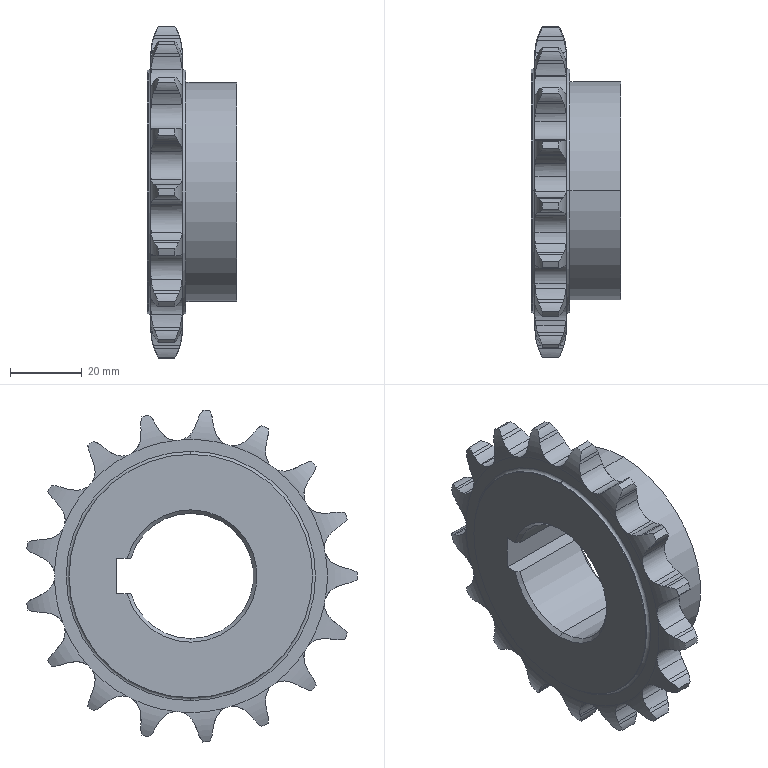Part | SolidWorks | features Chamfer 2, Cut 2, Revolution 2, CirPattern 1 | 1 solid | 207 faces | box 25 x 92.378 x 92.763 mm | volume 70331 mm3 | cylinder 119 | plane 42 | torus 40 | cone 6 | commonest cylinder face diameters 14.871 x36 26.567 x35 10.311 x22 93 x17 68 x4 35 x3